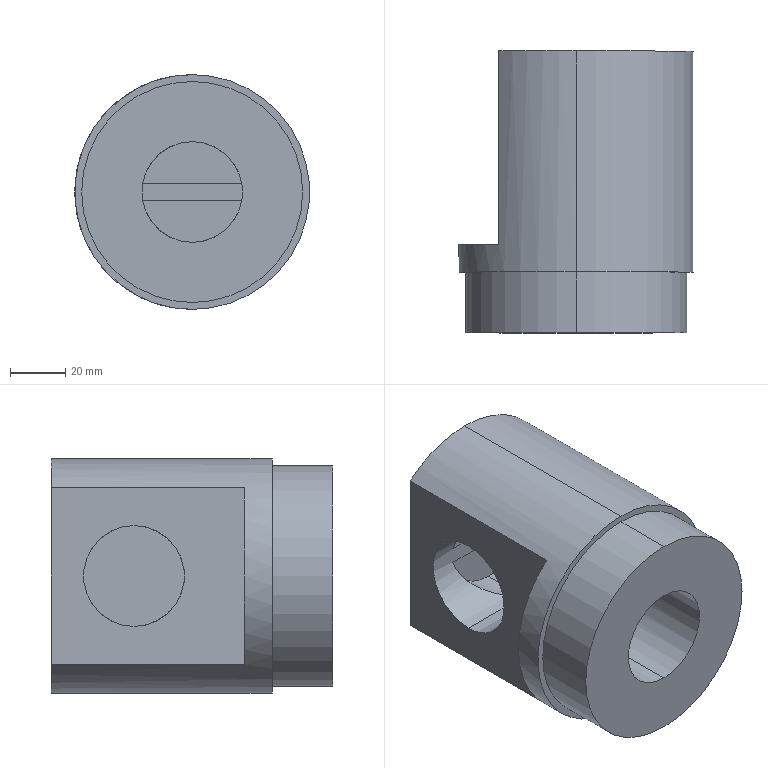Part | SolidWorks | features ICE 4, Extrusion 1 | 1 solid | 20 faces | box 85 x 102 x 85 mm | volume 399159 mm3 | cylinder 12 | plane 8 | commonest cylinder face diameters 36.5 x8 80 x2 85 x2
STEP:
#1=CARTESIAN_POINT('',(0.,90.,-18.25));
#2=VERTEX_POINT('',#1);
#3=CARTESIAN_POINT('',(18.,90.,-3.01));
#4=VERTEX_POINT('',#3);
#5=CARTESIAN_POINT('',(0.,90.,0.));
#6=DIRECTION('',(0.,-1.,0.));
#7=DIRECTION('',(0.,0.,-1.));
#8=AXIS2_PLACEMENT_3D('',#5,#6,#7);
#9=CIRCLE('',#8,18.25);
#10=EDGE_CURVE('',#2,#4,#9,.T.);
#11=ORIENTED_EDGE('',*,*,#10,.F.);
#12=CARTESIAN_POINT('',(0.,72.,-18.25));
#13=VERTEX_POINT('',#12);
#14=CARTESIAN_POINT('',(0.,90.,-18.25));
#15=DIRECTION('',(0.,-1.,0.));
#16=VECTOR('',#15,1000.);
#17=LINE('',#14,#16);
#18=EDGE_CURVE('',#2,#13,#17,.T.);
#19=ORIENTED_EDGE('',*,*,#18,.T.);
#20=CARTESIAN_POINT('',(0.,72.,-18.25));
#21=CARTESIAN_POINT('',(9.335,81.335,-18.25));
#22=CARTESIAN_POINT('',(16.46,88.46,-12.218));
#23=CARTESIAN_POINT('',(18.,90.,-3.01));
#24=(BOUNDED_CURVE()B_SPLINE_CURVE(3,(#20,#21,#22,#23),.UNSPECIFIED.,.F.,.F.)B_SPLINE_CURVE_WITH_KNOTS((4,4),(1.571,2.976),.UNSPECIFIED.)CURVE()GEOMETRIC_REPRESENTATION_ITEM()RATIONAL_B_SPLINE_CURVE((1.,0.8421,0.8421,1.))REPRESENTATION_ITEM(''));
#25=EDGE_CURVE('',#13,#4,#24,.T.);
#26=ORIENTED_EDGE('',*,*,#25,.T.);
#27=EDGE_LOOP('',(#11,#19,#26));
#28=FACE_OUTER_BOUND('',#27,.T.);
#29=CARTESIAN_POINT('',(0.,90.,0.));
#30=DIRECTION('',(0.,-1.,0.));
#31=DIRECTION('',(0.,0.,-1.));
#32=AXIS2_PLACEMENT_3D('',#29,#30,#31);
#33=CYLINDRICAL_SURFACE('',#32,18.25);
#34=ADVANCED_FACE('',(#28),#33,.F.);
#35=CARTESIAN_POINT('',(28.,72.,-18.25));
#36=VERTEX_POINT('',#35);
#37=CARTESIAN_POINT('',(28.,72.,18.25));
#38=VERTEX_POINT('',#37);
#39=CARTESIAN_POINT('',(28.,72.,0.));
#40=DIRECTION('',(-1.,0.,0.));
#41=DIRECTION('',(0.,0.,1.));
#42=AXIS2_PLACEMENT_3D('',#39,#40,#41);
#43=CIRCLE('',#42,18.25);
#44=EDGE_CURVE('',#36,#38,#43,.T.);
#45=ORIENTED_EDGE('',*,*,#44,.F.);
#46=CARTESIAN_POINT('',(28.,72.,-18.25));
#47=DIRECTION('',(-1.,0.,0.));
#48=VECTOR('',#47,1000.);
#49=LINE('',#46,#48);
#50=EDGE_CURVE('',#36,#13,#49,.T.);
#51=ORIENTED_EDGE('',*,*,#50,.T.);
#52=CARTESIAN_POINT('',(0.,72.,18.25));
#53=VERTEX_POINT('',#52);
#54=CARTESIAN_POINT('',(0.,72.,18.25));
#55=CARTESIAN_POINT('',(36.5,35.5,18.25));
#56=CARTESIAN_POINT('',(36.5,35.5,-18.25));
#57=CARTESIAN_POINT('',(0.,72.,-18.25));
#58=(BOUNDED_CURVE()B_SPLINE_CURVE(3,(#54,#55,#56,#57),.UNSPECIFIED.,.F.,.F.)B_SPLINE_CURVE_WITH_KNOTS((4,4),(4.712,7.854),.UNSPECIFIED.)CURVE()GEOMETRIC_REPRESENTATION_ITEM()RATIONAL_B_SPLINE_CURVE((1.,0.3333,0.3333,1.))REPRESENTATION_ITEM(''));
#59=EDGE_CURVE('',#53,#13,#58,.T.);
#60=ORIENTED_EDGE('',*,*,#59,.F.);
#61=CARTESIAN_POINT('',(28.,72.,18.25));
#62=DIRECTION('',(-1.,0.,0.));
#63=VECTOR('',#62,1000.);
#64=LINE('',#61,#63);
#65=EDGE_CURVE('',#38,#53,#64,.T.);
#66=ORIENTED_EDGE('',*,*,#65,.F.);
#67=EDGE_LOOP('',(#45,#51,#60,#66));
#68=FACE_OUTER_BOUND('',#67,.T.);
#69=CARTESIAN_POINT('',(28.,72.,0.));
#70=DIRECTION('',(-1.,0.,0.));
#71=DIRECTION('',(0.,0.,1.));
#72=AXIS2_PLACEMENT_3D('',#69,#70,#71);
#73=CYLINDRICAL_SURFACE('',#72,18.25);
#74=ADVANCED_FACE('',(#68),#73,.F.);
#75=CARTESIAN_POINT('',(0.,72.,-18.25));
#76=CARTESIAN_POINT('',(-36.5,35.5,-18.25));
#77=CARTESIAN_POINT('',(-36.5,35.5,18.25));
#78=CARTESIAN_POINT('',(0.,72.,18.25));
#79=(BOUNDED_CURVE()B_SPLINE_CURVE(3,(#75,#76,#77,#78),.UNSPECIFIED.,.F.,.F.)B_SPLINE_CURVE_WITH_KNOTS((4,4),(4.712,7.854),.UNSPECIFIED.)CURVE()GEOMETRIC_REPRESENTATION_ITEM()RATIONAL_B_SPLINE_CURVE((1.,0.3333,0.3333,1.))REPRESENTATION_ITEM(''));
#80=EDGE_CURVE('',#13,#53,#79,.T.);
#81=ORIENTED_EDGE('',*,*,#80,.F.);
#82=CARTESIAN_POINT('',(-28.,72.,-18.25));
#83=VERTEX_POINT('',#82);
#84=CARTESIAN_POINT('',(28.,72.,-18.25));
#85=DIRECTION('',(-1.,0.,0.));
#86=VECTOR('',#85,1000.);
#87=LINE('',#84,#86);
#88=EDGE_CURVE('',#13,#83,#87,.T.);
#89=ORIENTED_EDGE('',*,*,#88,.T.);
#90=CARTESIAN_POINT('',(-28.,72.,18.25));
#91=VERTEX_POINT('',#90);
#92=CARTESIAN_POINT('',(-28.,72.,0.));
#93=DIRECTION('',(-1.,0.,0.));
#94=DIRECTION('',(0.,0.,1.));
#95=AXIS2_PLACEMENT_3D('',#92,#93,#94);
#96=CIRCLE('',#95,18.25);
#97=EDGE_CURVE('',#83,#91,#96,.T.);
#98=ORIENTED_EDGE('',*,*,#97,.T.);
#99=CARTESIAN_POINT('',(28.,72.,18.25));
#100=DIRECTION('',(-1.,0.,0.));
#101=VECTOR('',#100,1000.);
#102=LINE('',#99,#101);
#103=EDGE_CURVE('',#53,#91,#102,.T.);
#104=ORIENTED_EDGE('',*,*,#103,.F.);
#105=EDGE_LOOP('',(#81,#89,#98,#104));
#106=FACE_OUTER_BOUND('',#105,.T.);
#107=CARTESIAN_POINT('',(28.,72.,0.));
#108=DIRECTION('',(-1.,0.,0.));
#109=DIRECTION('',(0.,0.,1.));
#110=AXIS2_PLACEMENT_3D('',#107,#108,#109);
#111=CYLINDRICAL_SURFACE('',#110,18.25);
#112=ADVANCED_FACE('',(#106),#111,.F.);
#113=CARTESIAN_POINT('',(0.,102.,42.5));
#114=VERTEX_POINT('',#113);
#115=CARTESIAN_POINT('',(0.,102.,-42.5));
#116=VERTEX_POINT('',#115);
#117=CARTESIAN_POINT('',(0.,102.,0.));
#118=DIRECTION('',(0.,1.,0.));
#119=DIRECTION('',(0.,0.,1.));
#120=AXIS2_PLACEMENT_3D('',#117,#118,#119);
#121=CIRCLE('',#120,42.5);
#122=EDGE_CURVE('',#114,#116,#121,.T.);
#123=ORIENTED_EDGE('',*,*,#122,.F.);
#124=CARTESIAN_POINT('',(0.,22.,42.5));
#125=VERTEX_POINT('',#124);
#126=CARTESIAN_POINT('',(0.,102.,42.5));
#127=DIRECTION('',(0.,-1.,0.));
#128=VECTOR('',#127,1000.);
#129=LINE('',#126,#128);
#130=EDGE_CURVE('',#114,#125,#129,.T.);
#131=ORIENTED_EDGE('',*,*,#130,.T.);
#132=CARTESIAN_POINT('',(0.,22.,-42.5));
#133=VERTEX_POINT('',#132);
#134=CARTESIAN_POINT('',(0.,22.,0.));
#135=DIRECTION('',(0.,1.,0.));
#136=DIRECTION('',(0.,0.,1.));
#137=AXIS2_PLACEMENT_3D('',#134,#135,#136);
#138=CIRCLE('',#137,42.5);
#139=EDGE_CURVE('',#125,#133,#138,.T.);
#140=ORIENTED_EDGE('',*,*,#139,.T.);
#141=CARTESIAN_POINT('',(0.,102.,-42.5));
#142=DIRECTION('',(0.,-1.,0.));
#143=VECTOR('',#142,1000.);
#144=LINE('',#141,#143);
#145=EDGE_CURVE('',#116,#133,#144,.T.);
#146=ORIENTED_EDGE('',*,*,#145,.F.);
#147=EDGE_LOOP('',(#123,#131,#140,#146));
#148=FACE_OUTER_BOUND('',#147,.T.);
#149=CARTESIAN_POINT('',(0.,102.,0.));
#150=DIRECTION('',(0.,-1.,0.));
#151=DIRECTION('',(0.,0.,-1.));
#152=AXIS2_PLACEMENT_3D('',#149,#150,#151);
#153=CYLINDRICAL_SURFACE('',#152,42.5);
#154=ADVANCED_FACE('',(#148),#153,.T.);
#155=CARTESIAN_POINT('',(0.,22.,40.));
#156=VERTEX_POINT('',#155);
#157=CARTESIAN_POINT('',(0.,22.,-40.));
#158=VERTEX_POINT('',#157);
#159=CARTESIAN_POINT('',(0.,22.,0.));
#160=DIRECTION('',(0.,1.,0.));
#161=DIRECTION('',(0.,0.,1.));
#162=AXIS2_PLACEMENT_3D('',#159,#160,#161);
#163=CIRCLE('',#162,40.);
#164=EDGE_CURVE('',#156,#158,#163,.T.);
#165=ORIENTED_EDGE('',*,*,#164,.F.);
#166=CARTESIAN_POINT('',(0.,0.,40.));
#167=VERTEX_POINT('',#166);
#168=CARTESIAN_POINT('',(0.,22.,40.));
#169=DIRECTION('',(0.,-1.,0.));
#170=VECTOR('',#169,1000.);
#171=LINE('',#168,#170);
#172=EDGE_CURVE('',#156,#167,#171,.T.);
#173=ORIENTED_EDGE('',*,*,#172,.T.);
#174=CARTESIAN_POINT('',(0.,0.,-40.));
#175=VERTEX_POINT('',#174);
#176=CARTESIAN_POINT('',(0.,0.,0.));
#177=DIRECTION('',(0.,1.,0.));
#178=DIRECTION('',(0.,0.,1.));
#179=AXIS2_PLACEMENT_3D('',#176,#177,#178);
#180=CIRCLE('',#179,40.);
#181=EDGE_CURVE('',#167,#175,#180,.T.);
#182=ORIENTED_EDGE('',*,*,#181,.T.);
#183=CARTESIAN_POINT('',(0.,22.,-40.));
#184=DIRECTION('',(0.,-1.,0.));
#185=VECTOR('',#184,1000.);
#186=LINE('',#183,#185);
#187=EDGE_CURVE('',#158,#175,#186,.T.);
#188=ORIENTED_EDGE('',*,*,#187,.F.);
#189=EDGE_LOOP('',(#165,#173,#182,#188));
#190=FACE_OUTER_BOUND('',#189,.T.);
#191=CARTESIAN_POINT('',(0.,22.,0.));
#192=DIRECTION('',(0.,-1.,0.));
#193=DIRECTION('',(0.,0.,-1.));
#194=AXIS2_PLACEMENT_3D('',#191,#192,#193);
#195=CYLINDRICAL_SURFACE('',#194,40.);
#196=ADVANCED_FACE('',(#190),#195,.T.);
#197=ORIENTED_EDGE('',*,*,#80,.T.);
#198=CARTESIAN_POINT('',(0.,0.,18.25));
#199=VERTEX_POINT('',#198);
#200=CARTESIAN_POINT('',(0.,90.,18.25));
#201=DIRECTION('',(0.,-1.,0.));
#202=VECTOR('',#201,1000.);
#203=LINE('',#200,#202);
#204=EDGE_CURVE('',#53,#199,#203,.T.);
#205=ORIENTED_EDGE('',*,*,#204,.T.);
#206=CARTESIAN_POINT('',(0.,0.,-18.25));
#207=VERTEX_POINT('',#206);
#208=CARTESIAN_POINT('',(0.,0.,0.));
#209=DIRECTION('',(0.,-1.,0.));
#210=DIRECTION('',(0.,0.,-1.));
#211=AXIS2_PLACEMENT_3D('',#208,#209,#210);
#212=CIRCLE('',#211,18.25);
#213=EDGE_CURVE('',#199,#207,#212,.T.);
#214=ORIENTED_EDGE('',*,*,#213,.T.);
#215=CARTESIAN_POINT('',(0.,90.,-18.25));
#216=DIRECTION('',(0.,-1.,0.));
#217=VECTOR('',#216,1000.);
#218=LINE('',#215,#217);
#219=EDGE_CURVE('',#13,#207,#218,.T.);
#220=ORIENTED_EDGE('',*,*,#219,.F.);
#221=EDGE_LOOP('',(#197,#205,#214,#220));
#222=FACE_OUTER_BOUND('',#221,.T.);
#223=CARTESIAN_POINT('',(0.,90.,0.));
#224=DIRECTION('',(0.,-1.,0.));
#225=DIRECTION('',(0.,0.,-1.));
#226=AXIS2_PLACEMENT_3D('',#223,#224,#225);
#227=CYLINDRICAL_SURFACE('',#226,18.25);
#228=ADVANCED_FACE('',(#222),#227,.F.);
#229=ORIENTED_EDGE('',*,*,#204,.F.);
#230=ORIENTED_EDGE('',*,*,#59,.T.);
#231=ORIENTED_EDGE('',*,*,#219,.T.);
#232=CARTESIAN_POINT('',(0.,0.,0.));
#233=DIRECTION('',(0.,-1.,0.));
#234=DIRECTION('',(0.,0.,-1.));
#235=AXIS2_PLACEMENT_3D('',#232,#233,#234);
#236=CIRCLE('',#235,18.25);
#237=EDGE_CURVE('',#207,#199,#236,.T.);
#238=ORIENTED_EDGE('',*,*,#237,.T.);
#239=EDGE_LOOP('',(#229,#230,#231,#238));
#240=FACE_OUTER_BOUND('',#239,.T.);
#241=CARTESIAN_POINT('',(0.,90.,0.));
#242=DIRECTION('',(0.,-1.,0.));
#243=DIRECTION('',(0.,0.,-1.));
#244=AXIS2_PLACEMENT_3D('',#241,#242,#243);
#245=CYLINDRICAL_SURFACE('',#244,18.25);
#246=ADVANCED_FACE('',(#240),#245,.F.);
#247=ORIENTED_EDGE('',*,*,#172,.F.);
#248=CARTESIAN_POINT('',(0.,22.,0.));
#249=DIRECTION('',(0.,1.,0.));
#250=DIRECTION('',(0.,0.,1.));
#251=AXIS2_PLACEMENT_3D('',#248,#249,#250);
#252=CIRCLE('',#251,40.);
#253=EDGE_CURVE('',#158,#156,#252,.T.);
#254=ORIENTED_EDGE('',*,*,#253,.F.);
#255=ORIENTED_EDGE('',*,*,#187,.T.);
#256=CARTESIAN_POINT('',(0.,0.,0.));
#257=DIRECTION('',(0.,1.,0.));
#258=DIRECTION('',(0.,0.,1.));
#259=AXIS2_PLACEMENT_3D('',#256,#257,#258);
#260=CIRCLE('',#259,40.);
#261=EDGE_CURVE('',#175,#167,#260,.T.);
#262=ORIENTED_EDGE('',*,*,#261,.T.);
#263=EDGE_LOOP('',(#247,#254,#255,#262));
#264=FACE_OUTER_BOUND('',#263,.T.);
#265=CARTESIAN_POINT('',(0.,22.,0.));
#266=DIRECTION('',(0.,-1.,0.));
#267=DIRECTION('',(0.,0.,-1.));
#268=AXIS2_PLACEMENT_3D('',#265,#266,#267);
#269=CYLINDRICAL_SURFACE('',#268,40.);
#270=ADVANCED_FACE('',(#264),#269,.T.);
#271=ORIENTED_EDGE('',*,*,#237,.F.);
#272=ORIENTED_EDGE('',*,*,#213,.F.);
#273=EDGE_LOOP('',(#271,#272));
#274=FACE_BOUND('',#273,.T.);
#275=ORIENTED_EDGE('',*,*,#261,.F.);
#276=ORIENTED_EDGE('',*,*,#181,.F.);
#277=EDGE_LOOP('',(#275,#276));
#278=FACE_OUTER_BOUND('',#277,.T.);
#279=CARTESIAN_POINT('',(0.,0.,0.));
#280=DIRECTION('',(0.,1.,0.));
#281=DIRECTION('',(0.,0.,1.));
#282=AXIS2_PLACEMENT_3D('',#279,#280,#281);
#283=PLANE('',#282);
#284=ADVANCED_FACE('',(#274,#278),#283,.F.);
#285=ORIENTED_EDGE('',*,*,#130,.F.);
#286=CARTESIAN_POINT('',(-28.,102.,31.973));
#287=VERTEX_POINT('',#286);
#288=CARTESIAN_POINT('',(0.,102.,0.));
#289=DIRECTION('',(0.,1.,0.));
#290=DIRECTION('',(0.,0.,1.));
#291=AXIS2_PLACEMENT_3D('',#288,#289,#290);
#292=CIRCLE('',#291,42.5);
#293=EDGE_CURVE('',#287,#114,#292,.T.);
#294=ORIENTED_EDGE('',*,*,#293,.F.);
#295=CARTESIAN_POINT('',(-28.,32.,31.973));
#296=VERTEX_POINT('',#295);
#297=CARTESIAN_POINT('',(-28.,102.,31.973));
#298=DIRECTION('',(0.,-1.,0.));
#299=VECTOR('',#298,1000.);
#300=LINE('',#297,#299);
#301=EDGE_CURVE('',#287,#296,#300,.T.);
#302=ORIENTED_EDGE('',*,*,#301,.T.);
#303=CARTESIAN_POINT('',(-28.,32.,-31.973));
#304=VERTEX_POINT('',#303);
#305=CARTESIAN_POINT('',(0.,32.,0.));
#306=DIRECTION('',(0.,-1.,0.));
#307=DIRECTION('',(0.,0.,-1.));
#308=AXIS2_PLACEMENT_3D('',#305,#306,#307);
#309=CIRCLE('',#308,42.5);
#310=EDGE_CURVE('',#296,#304,#309,.T.);
#311=ORIENTED_EDGE('',*,*,#310,.T.);
#312=CARTESIAN_POINT('',(-28.,102.,-31.973));
#313=VERTEX_POINT('',#312);
#314=CARTESIAN_POINT('',(-28.,102.,-31.973));
#315=DIRECTION('',(0.,1.,0.));
#316=VECTOR('',#315,1000.);
#317=LINE('',#314,#316);
#318=EDGE_CURVE('',#304,#313,#317,.T.);
#319=ORIENTED_EDGE('',*,*,#318,.T.);
#320=CARTESIAN_POINT('',(0.,102.,0.));
#321=DIRECTION('',(0.,1.,0.));
#322=DIRECTION('',(0.,0.,1.));
#323=AXIS2_PLACEMENT_3D('',#320,#321,#322);
#324=CIRCLE('',#323,42.5);
#325=EDGE_CURVE('',#116,#313,#324,.T.);
#326=ORIENTED_EDGE('',*,*,#325,.F.);
#327=ORIENTED_EDGE('',*,*,#145,.T.);
#328=CARTESIAN_POINT('',(0.,22.,0.));
#329=DIRECTION('',(0.,1.,0.));
#330=DIRECTION('',(0.,0.,1.));
#331=AXIS2_PLACEMENT_3D('',#328,#329,#330);
#332=CIRCLE('',#331,42.5);
#333=EDGE_CURVE('',#133,#125,#332,.T.);
#334=ORIENTED_EDGE('',*,*,#333,.T.);
#335=EDGE_LOOP('',(#285,#294,#302,#311,#319,#326,#327,#334));
#336=FACE_OUTER_BOUND('',#335,.T.);
#337=CARTESIAN_POINT('',(0.,102.,0.));
#338=DIRECTION('',(0.,-1.,0.));
#339=DIRECTION('',(0.,0.,-1.));
#340=AXIS2_PLACEMENT_3D('',#337,#338,#339);
#341=CYLINDRICAL_SURFACE('',#340,42.5);
#342=ADVANCED_FACE('',(#336),#341,.T.);
#343=CARTESIAN_POINT('',(-28.,102.,0.));
#344=DIRECTION('',(0.,0.,-1.));
#345=VECTOR('',#344,1000.);
#346=LINE('',#343,#345);
#347=EDGE_CURVE('',#287,#313,#346,.T.);
#348=ORIENTED_EDGE('',*,*,#347,.F.);
#349=ORIENTED_EDGE('',*,*,#293,.T.);
#350=ORIENTED_EDGE('',*,*,#122,.T.);
#351=ORIENTED_EDGE('',*,*,#325,.T.);
#352=EDGE_LOOP('',(#348,#349,#350,#351));
#353=FACE_OUTER_BOUND('',#352,.T.);
#354=CARTESIAN_POINT('',(0.,102.,0.));
#355=DIRECTION('',(0.,1.,0.));
#356=DIRECTION('',(0.,0.,1.));
#357=AXIS2_PLACEMENT_3D('',#354,#355,#356);
#358=PLANE('',#357);
#359=ADVANCED_FACE('',(#353),#358,.T.);
#360=ORIENTED_EDGE('',*,*,#253,.T.);
#361=ORIENTED_EDGE('',*,*,#164,.T.);
#362=EDGE_LOOP('',(#360,#361));
#363=FACE_BOUND('',#362,.T.);
#364=ORIENTED_EDGE('',*,*,#333,.F.);
#365=ORIENTED_EDGE('',*,*,#139,.F.);
#366=EDGE_LOOP('',(#364,#365));
#367=FACE_OUTER_BOUND('',#366,.T.);
#368=CARTESIAN_POINT('',(0.,22.,0.));
#369=DIRECTION('',(0.,1.,0.));
#370=DIRECTION('',(0.,0.,1.));
#371=AXIS2_PLACEMENT_3D('',#368,#369,#370);
#372=PLANE('',#371);
#373=ADVANCED_FACE('',(#363,#367),#372,.F.);
#374=CARTESIAN_POINT('',(-28.,32.,32.5));
#375=DIRECTION('',(0.,0.,-1.));
#376=VECTOR('',#375,1000.);
#377=LINE('',#374,#376);
#378=EDGE_CURVE('',#296,#304,#377,.T.);
#379=ORIENTED_EDGE('',*,*,#378,.T.);
#380=ORIENTED_EDGE('',*,*,#310,.F.);
#381=EDGE_LOOP('',(#379,#380));
#382=FACE_OUTER_BOUND('',#381,.T.);
#383=CARTESIAN_POINT('',(-108.,32.,32.5));
#384=DIRECTION('',(0.,-1.,0.));
#385=DIRECTION('',(0.,0.,-1.));
#386=AXIS2_PLACEMENT_3D('',#383,#384,#385);
#387=PLANE('',#386);
#388=ADVANCED_FACE('',(#382),#387,.F.);
#389=CARTESIAN_POINT('',(-28.,72.,0.));
#390=DIRECTION('',(-1.,0.,0.));
#391=DIRECTION('',(0.,0.,1.));
#392=AXIS2_PLACEMENT_3D('',#389,#390,#391);
#393=CIRCLE('',#392,18.25);
#394=EDGE_CURVE('',#91,#83,#393,.T.);
#395=ORIENTED_EDGE('',*,*,#394,.F.);
#396=ORIENTED_EDGE('',*,*,#97,.F.);
#397=EDGE_LOOP('',(#395,#396));
#398=FACE_BOUND('',#397,.T.);
#399=ORIENTED_EDGE('',*,*,#347,.T.);
#400=ORIENTED_EDGE('',*,*,#318,.F.);
#401=ORIENTED_EDGE('',*,*,#378,.F.);
#402=ORIENTED_EDGE('',*,*,#301,.F.);
#403=EDGE_LOOP('',(#399,#400,#401,#402));
#404=FACE_OUTER_BOUND('',#403,.T.);
#405=CARTESIAN_POINT('',(-28.,0.,0.));
#406=DIRECTION('',(1.,0.,0.));
#407=DIRECTION('',(0.,0.,-1.));
#408=AXIS2_PLACEMENT_3D('',#405,#406,#407);
#409=PLANE('',#408);
#410=ADVANCED_FACE('',(#398,#404),#409,.F.);
#411=ORIENTED_EDGE('',*,*,#50,.F.);
#412=CARTESIAN_POINT('',(28.,72.,0.));
#413=DIRECTION('',(-1.,0.,0.));
#414=DIRECTION('',(0.,0.,1.));
#415=AXIS2_PLACEMENT_3D('',#412,#413,#414);
#416=CIRCLE('',#415,18.25);
#417=EDGE_CURVE('',#38,#36,#416,.T.);
#418=ORIENTED_EDGE('',*,*,#417,.F.);
#419=ORIENTED_EDGE('',*,*,#65,.T.);
#420=CARTESIAN_POINT('',(18.,90.,3.01));
#421=VERTEX_POINT('',#420);
#422=CARTESIAN_POINT('',(18.,90.,3.01));
#423=CARTESIAN_POINT('',(16.46,88.46,12.218));
#424=CARTESIAN_POINT('',(9.335,81.335,18.25));
#425=CARTESIAN_POINT('',(0.,72.,18.25));
#426=(BOUNDED_CURVE()B_SPLINE_CURVE(3,(#422,#423,#424,#425),.UNSPECIFIED.,.F.,.T.)B_SPLINE_CURVE_WITH_KNOTS((4,4),(3.307,4.712),.UNSPECIFIED.)CURVE()GEOMETRIC_REPRESENTATION_ITEM()RATIONAL_B_SPLINE_CURVE((1.,0.8421,0.8421,1.))REPRESENTATION_ITEM(''));
#427=EDGE_CURVE('',#421,#53,#426,.T.);
#428=ORIENTED_EDGE('',*,*,#427,.F.);
#429=CARTESIAN_POINT('',(-18.,90.,3.01));
#430=VERTEX_POINT('',#429);
#431=CARTESIAN_POINT('',(28.,90.,3.01));
#432=DIRECTION('',(-1.,0.,0.));
#433=VECTOR('',#432,1000.);
#434=LINE('',#431,#433);
#435=EDGE_CURVE('',#421,#430,#434,.T.);
#436=ORIENTED_EDGE('',*,*,#435,.T.);
#437=CARTESIAN_POINT('',(0.,72.,18.25));
#438=CARTESIAN_POINT('',(-9.335,81.335,18.25));
#439=CARTESIAN_POINT('',(-16.46,88.46,12.218));
#440=CARTESIAN_POINT('',(-18.,90.,3.01));
#441=(BOUNDED_CURVE()B_SPLINE_CURVE(3,(#437,#438,#439,#440),.UNSPECIFIED.,.F.,.T.)B_SPLINE_CURVE_WITH_KNOTS((4,4),(1.571,2.976),.UNSPECIFIED.)CURVE()GEOMETRIC_REPRESENTATION_ITEM()RATIONAL_B_SPLINE_CURVE((1.,0.8421,0.8421,1.))REPRESENTATION_ITEM(''));
#442=EDGE_CURVE('',#53,#430,#441,.T.);
#443=ORIENTED_EDGE('',*,*,#442,.F.);
#444=ORIENTED_EDGE('',*,*,#103,.T.);
#445=ORIENTED_EDGE('',*,*,#394,.T.);
#446=ORIENTED_EDGE('',*,*,#88,.F.);
#447=CARTESIAN_POINT('',(-18.,90.,-3.01));
#448=VERTEX_POINT('',#447);
#449=CARTESIAN_POINT('',(-18.,90.,-3.01));
#450=CARTESIAN_POINT('',(-16.46,88.46,-12.218));
#451=CARTESIAN_POINT('',(-9.335,81.335,-18.25));
#452=CARTESIAN_POINT('',(0.,72.,-18.25));
#453=(BOUNDED_CURVE()B_SPLINE_CURVE(3,(#449,#450,#451,#452),.UNSPECIFIED.,.F.,.F.)B_SPLINE_CURVE_WITH_KNOTS((4,4),(3.307,4.712),.UNSPECIFIED.)CURVE()GEOMETRIC_REPRESENTATION_ITEM()RATIONAL_B_SPLINE_CURVE((1.,0.8421,0.8421,1.))REPRESENTATION_ITEM(''));
#454=EDGE_CURVE('',#448,#13,#453,.T.);
#455=ORIENTED_EDGE('',*,*,#454,.F.);
#456=CARTESIAN_POINT('',(28.,90.,-3.01));
#457=DIRECTION('',(1.,0.,0.));
#458=VECTOR('',#457,1000.);
#459=LINE('',#456,#458);
#460=EDGE_CURVE('',#448,#4,#459,.T.);
#461=ORIENTED_EDGE('',*,*,#460,.T.);
#462=ORIENTED_EDGE('',*,*,#25,.F.);
#463=EDGE_LOOP('',(#411,#418,#419,#428,#436,#443,#444,#445,#446,#455,#461,#462));
#464=FACE_OUTER_BOUND('',#463,.T.);
#465=CARTESIAN_POINT('',(28.,72.,0.));
#466=DIRECTION('',(-1.,0.,0.));
#467=DIRECTION('',(0.,0.,1.));
#468=AXIS2_PLACEMENT_3D('',#465,#466,#467);
#469=CYLINDRICAL_SURFACE('',#468,18.25);
#470=ADVANCED_FACE('',(#464),#469,.F.);
#471=ORIENTED_EDGE('',*,*,#417,.T.);
#472=ORIENTED_EDGE('',*,*,#44,.T.);
#473=EDGE_LOOP('',(#471,#472));
#474=FACE_OUTER_BOUND('',#473,.T.);
#475=CARTESIAN_POINT('',(28.,72.,0.));
#476=DIRECTION('',(-1.,0.,0.));
#477=DIRECTION('',(0.,0.,1.));
#478=AXIS2_PLACEMENT_3D('',#475,#476,#477);
#479=PLANE('',#478);
#480=ADVANCED_FACE('',(#474),#479,.T.);
#481=ORIENTED_EDGE('',*,*,#435,.F.);
#482=CARTESIAN_POINT('',(0.,90.,0.));
#483=DIRECTION('',(0.,-1.,0.));
#484=DIRECTION('',(0.,0.,-1.));
#485=AXIS2_PLACEMENT_3D('',#482,#483,#484);
#486=CIRCLE('',#485,18.25);
#487=EDGE_CURVE('',#421,#430,#486,.T.);
#488=ORIENTED_EDGE('',*,*,#487,.T.);
#489=EDGE_LOOP('',(#481,#488));
#490=FACE_OUTER_BOUND('',#489,.T.);
#491=CARTESIAN_POINT('',(0.,90.,0.));
#492=DIRECTION('',(0.,-1.,0.));
#493=DIRECTION('',(0.,0.,-1.));
#494=AXIS2_PLACEMENT_3D('',#491,#492,#493);
#495=PLANE('',#494);
#496=ADVANCED_FACE('',(#490),#495,.T.);
#497=ORIENTED_EDGE('',*,*,#427,.T.);
#498=ORIENTED_EDGE('',*,*,#442,.T.);
#499=ORIENTED_EDGE('',*,*,#487,.F.);
#500=EDGE_LOOP('',(#497,#498,#499));
#501=FACE_OUTER_BOUND('',#500,.T.);
#502=CARTESIAN_POINT('',(0.,90.,0.));
#503=DIRECTION('',(0.,-1.,0.));
#504=DIRECTION('',(0.,0.,-1.));
#505=AXIS2_PLACEMENT_3D('',#502,#503,#504);
#506=CYLINDRICAL_SURFACE('',#505,18.25);
#507=ADVANCED_FACE('',(#501),#506,.F.);
#508=ORIENTED_EDGE('',*,*,#460,.F.);
#509=CARTESIAN_POINT('',(0.,90.,0.));
#510=DIRECTION('',(0.,-1.,0.));
#511=DIRECTION('',(0.,0.,-1.));
#512=AXIS2_PLACEMENT_3D('',#509,#510,#511);
#513=CIRCLE('',#512,18.25);
#514=EDGE_CURVE('',#448,#2,#513,.T.);
#515=ORIENTED_EDGE('',*,*,#514,.T.);
#516=ORIENTED_EDGE('',*,*,#10,.T.);
#517=EDGE_LOOP('',(#508,#515,#516));
#518=FACE_OUTER_BOUND('',#517,.T.);
#519=CARTESIAN_POINT('',(0.,90.,0.));
#520=DIRECTION('',(0.,-1.,0.));
#521=DIRECTION('',(0.,0.,-1.));
#522=AXIS2_PLACEMENT_3D('',#519,#520,#521);
#523=PLANE('',#522);
#524=ADVANCED_FACE('',(#518),#523,.T.);
#525=ORIENTED_EDGE('',*,*,#18,.F.);
#526=ORIENTED_EDGE('',*,*,#514,.F.);
#527=ORIENTED_EDGE('',*,*,#454,.T.);
#528=EDGE_LOOP('',(#525,#526,#527));
#529=FACE_OUTER_BOUND('',#528,.T.);
#530=CARTESIAN_POINT('',(0.,90.,0.));
#531=DIRECTION('',(0.,-1.,0.));
#532=DIRECTION('',(0.,0.,-1.));
#533=AXIS2_PLACEMENT_3D('',#530,#531,#532);
#534=CYLINDRICAL_SURFACE('',#533,18.25);
#535=ADVANCED_FACE('',(#529),#534,.F.);
#536=CLOSED_SHELL('',(#34,#74,#112,#154,#196,#228,#246,#270,#284,#342,#359,#373,#388,#410,#470,#480,#496,#507,#524,#535));
#537=MANIFOLD_SOLID_BREP('',#536);
#538=CARTESIAN_POINT('',(0.,0.,0.));
#539=DIRECTION('',(0.,0.,1.));
#540=DIRECTION('',(1.,0.,0.));
#541=AXIS2_PLACEMENT_3D('',#538,#539,#540);
#542=(LENGTH_UNIT()NAMED_UNIT(*)SI_UNIT(.MILLI.,.METRE.));
#543=UNCERTAINTY_MEASURE_WITH_UNIT(LENGTH_MEASURE(0.00001),#542,'','');
#544=(NAMED_UNIT(*)PLANE_ANGLE_UNIT()SI_UNIT($,.RADIAN.));
#545=(NAMED_UNIT(*)SI_UNIT($,.STERADIAN.)SOLID_ANGLE_UNIT());
#546=(GEOMETRIC_REPRESENTATION_CONTEXT(3)GLOBAL_UNCERTAINTY_ASSIGNED_CONTEXT((#543))GLOBAL_UNIT_ASSIGNED_CONTEXT((#542,#544,#545))REPRESENTATION_CONTEXT('',''));
#547=ADVANCED_BREP_SHAPE_REPRESENTATION('',(#537,#541),#546);